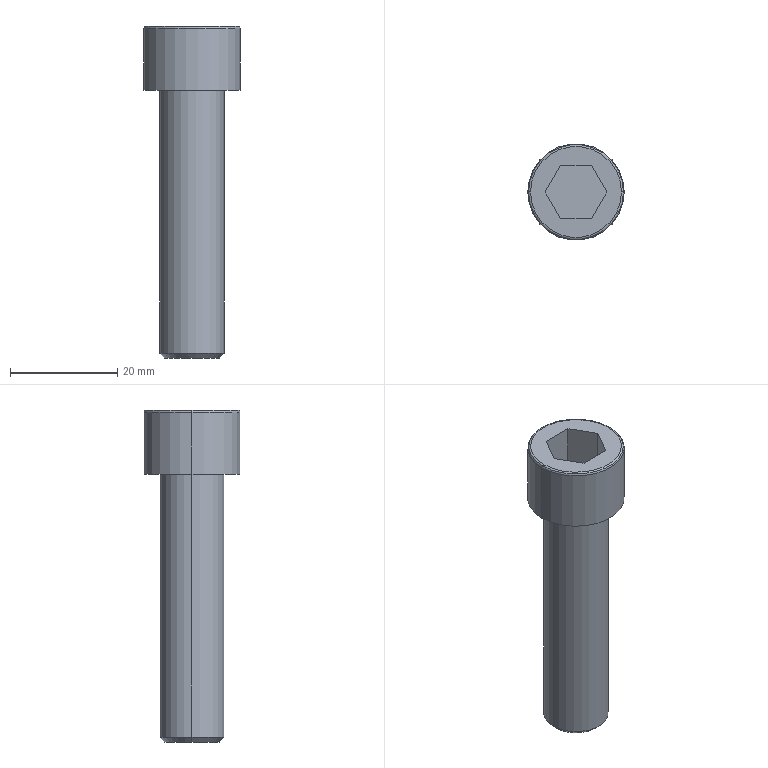Part | Creo | 1 solid | 20 faces | box 18 x 18 x 62 mm | volume 8005 mm3 | plane 10 | torus 4 | cylinder 4 | cone 2 | commonest cylinder face diameters 12 x2 18 x2
STEP:
#1=CARTESIAN_POINT('',(198.5,250.,159.5));
#2=VERTEX_POINT('',#1);
#3=CARTESIAN_POINT('',(181.5,250.,159.5));
#4=VERTEX_POINT('',#3);
#5=CARTESIAN_POINT('',(190.,250.,159.5));
#6=DIRECTION('',(0.,0.,1.));
#7=DIRECTION('',(1.,0.,0.));
#8=AXIS2_PLACEMENT_3D('',#5,#6,#7);
#9=CIRCLE('',#8,8.5);
#10=EDGE_CURVE('',#2,#4,#9,.T.);
#11=ORIENTED_EDGE('',*,*,#10,.F.);
#12=CARTESIAN_POINT('',(190.,250.,159.5));
#13=DIRECTION('',(0.,0.,1.));
#14=DIRECTION('',(-1.,0.,0.));
#15=AXIS2_PLACEMENT_3D('',#12,#13,#14);
#16=CIRCLE('',#15,8.5);
#17=EDGE_CURVE('',#4,#2,#16,.T.);
#18=ORIENTED_EDGE('',*,*,#17,.F.);
#19=EDGE_LOOP('',(#11,#18));
#20=FACE_OUTER_BOUND('',#19,.F.);
#21=CARTESIAN_POINT('',(192.887,255.,159.5));
#22=VERTEX_POINT('',#21);
#23=CARTESIAN_POINT('',(187.113,255.,159.5));
#24=VERTEX_POINT('',#23);
#25=CARTESIAN_POINT('',(192.887,255.,159.5));
#26=DIRECTION('',(-1.,0.,0.));
#27=VECTOR('',#26,5.774);
#28=LINE('',#25,#27);
#29=EDGE_CURVE('',#22,#24,#28,.T.);
#30=ORIENTED_EDGE('',*,*,#29,.T.);
#31=CARTESIAN_POINT('',(184.226,250.,159.5));
#32=VERTEX_POINT('',#31);
#33=CARTESIAN_POINT('',(184.226,250.,159.5));
#34=DIRECTION('',(0.5,0.866,0.));
#35=VECTOR('',#34,5.774);
#36=LINE('',#33,#35);
#37=EDGE_CURVE('',#32,#24,#36,.T.);
#38=ORIENTED_EDGE('',*,*,#37,.F.);
#39=CARTESIAN_POINT('',(187.113,245.,159.5));
#40=VERTEX_POINT('',#39);
#41=CARTESIAN_POINT('',(187.113,245.,159.5));
#42=DIRECTION('',(-0.5,0.866,0.));
#43=VECTOR('',#42,5.774);
#44=LINE('',#41,#43);
#45=EDGE_CURVE('',#40,#32,#44,.T.);
#46=ORIENTED_EDGE('',*,*,#45,.F.);
#47=CARTESIAN_POINT('',(192.887,245.,159.5));
#48=VERTEX_POINT('',#47);
#49=CARTESIAN_POINT('',(187.113,245.,159.5));
#50=DIRECTION('',(1.,0.,0.));
#51=VECTOR('',#50,5.774);
#52=LINE('',#49,#51);
#53=EDGE_CURVE('',#40,#48,#52,.T.);
#54=ORIENTED_EDGE('',*,*,#53,.T.);
#55=CARTESIAN_POINT('',(195.774,250.,159.5));
#56=VERTEX_POINT('',#55);
#57=CARTESIAN_POINT('',(195.774,250.,159.5));
#58=DIRECTION('',(-0.5,-0.866,0.));
#59=VECTOR('',#58,5.774);
#60=LINE('',#57,#59);
#61=EDGE_CURVE('',#56,#48,#60,.T.);
#62=ORIENTED_EDGE('',*,*,#61,.F.);
#63=CARTESIAN_POINT('',(192.887,255.,159.5));
#64=DIRECTION('',(0.5,-0.866,0.));
#65=VECTOR('',#64,5.774);
#66=LINE('',#63,#65);
#67=EDGE_CURVE('',#22,#56,#66,.T.);
#68=ORIENTED_EDGE('',*,*,#67,.F.);
#69=EDGE_LOOP('',(#30,#38,#46,#54,#62,#68));
#70=FACE_BOUND('',#69,.F.);
#71=CARTESIAN_POINT('',(190.,250.,159.5));
#72=DIRECTION('',(0.,0.,1.));
#73=DIRECTION('',(1.,0.,0.));
#74=AXIS2_PLACEMENT_3D('',#71,#72,#73);
#75=PLANE('',#74);
#76=ADVANCED_FACE('',(#20,#70),#75,.T.);
#77=ORIENTED_EDGE('',*,*,#10,.T.);
#78=CARTESIAN_POINT('',(181.146,250.,159.354));
#79=VERTEX_POINT('',#78);
#80=CARTESIAN_POINT('',(181.5,250.,159.));
#81=DIRECTION('',(0.,1.,0.));
#82=DIRECTION('',(-0.7071,0.,0.7071));
#83=AXIS2_PLACEMENT_3D('',#80,#81,#82);
#84=CIRCLE('',#83,0.5);
#85=EDGE_CURVE('',#79,#4,#84,.T.);
#86=ORIENTED_EDGE('',*,*,#85,.F.);
#87=CARTESIAN_POINT('',(198.854,250.,159.354));
#88=VERTEX_POINT('',#87);
#89=CARTESIAN_POINT('',(190.,250.,159.354));
#90=DIRECTION('',(0.,0.,1.));
#91=DIRECTION('',(1.,0.,0.));
#92=AXIS2_PLACEMENT_3D('',#89,#90,#91);
#93=CIRCLE('',#92,8.854);
#94=EDGE_CURVE('',#88,#79,#93,.T.);
#95=ORIENTED_EDGE('',*,*,#94,.F.);
#96=CARTESIAN_POINT('',(198.5,250.,159.));
#97=DIRECTION('',(0.,-1.,0.));
#98=DIRECTION('',(0.7071,0.,0.7071));
#99=AXIS2_PLACEMENT_3D('',#96,#97,#98);
#100=CIRCLE('',#99,0.5);
#101=EDGE_CURVE('',#88,#2,#100,.T.);
#102=ORIENTED_EDGE('',*,*,#101,.T.);
#103=EDGE_LOOP('',(#77,#86,#95,#102));
#104=FACE_OUTER_BOUND('',#103,.F.);
#105=CARTESIAN_POINT('',(190.,250.,159.));
#106=DIRECTION('',(0.,0.,1.));
#107=DIRECTION('',(1.,0.,0.));
#108=AXIS2_PLACEMENT_3D('',#105,#106,#107);
#109=TOROIDAL_SURFACE('',#108,8.5,0.5);
#110=ADVANCED_FACE('',(#104),#109,.T.);
#111=ORIENTED_EDGE('',*,*,#17,.T.);
#112=ORIENTED_EDGE('',*,*,#101,.F.);
#113=CARTESIAN_POINT('',(190.,250.,159.354));
#114=DIRECTION('',(0.,0.,1.));
#115=DIRECTION('',(-1.,0.,0.));
#116=AXIS2_PLACEMENT_3D('',#113,#114,#115);
#117=CIRCLE('',#116,8.854);
#118=EDGE_CURVE('',#79,#88,#117,.T.);
#119=ORIENTED_EDGE('',*,*,#118,.F.);
#120=ORIENTED_EDGE('',*,*,#85,.T.);
#121=EDGE_LOOP('',(#111,#112,#119,#120));
#122=FACE_OUTER_BOUND('',#121,.F.);
#123=CARTESIAN_POINT('',(190.,250.,159.));
#124=DIRECTION('',(0.,0.,1.));
#125=DIRECTION('',(1.,0.,0.));
#126=AXIS2_PLACEMENT_3D('',#123,#124,#125);
#127=TOROIDAL_SURFACE('',#126,8.5,0.5);
#128=ADVANCED_FACE('',(#122),#127,.T.);
#129=CARTESIAN_POINT('',(181.,250.,159.));
#130=VERTEX_POINT('',#129);
#131=CARTESIAN_POINT('',(199.,250.,159.));
#132=VERTEX_POINT('',#131);
#133=CARTESIAN_POINT('',(190.,250.,159.));
#134=DIRECTION('',(0.,0.,1.));
#135=DIRECTION('',(-1.,0.,0.));
#136=AXIS2_PLACEMENT_3D('',#133,#134,#135);
#137=CIRCLE('',#136,9.);
#138=EDGE_CURVE('',#130,#132,#137,.T.);
#139=ORIENTED_EDGE('',*,*,#138,.F.);
#140=CARTESIAN_POINT('',(181.5,250.,159.));
#141=DIRECTION('',(0.,1.,0.));
#142=DIRECTION('',(-1.,0.,0.));
#143=AXIS2_PLACEMENT_3D('',#140,#141,#142);
#144=CIRCLE('',#143,0.5);
#145=EDGE_CURVE('',#130,#79,#144,.T.);
#146=ORIENTED_EDGE('',*,*,#145,.T.);
#147=ORIENTED_EDGE('',*,*,#118,.T.);
#148=CARTESIAN_POINT('',(198.5,250.,159.));
#149=DIRECTION('',(0.,-1.,0.));
#150=DIRECTION('',(1.,0.,0.));
#151=AXIS2_PLACEMENT_3D('',#148,#149,#150);
#152=CIRCLE('',#151,0.5);
#153=EDGE_CURVE('',#132,#88,#152,.T.);
#154=ORIENTED_EDGE('',*,*,#153,.F.);
#155=EDGE_LOOP('',(#139,#146,#147,#154));
#156=FACE_OUTER_BOUND('',#155,.F.);
#157=CARTESIAN_POINT('',(190.,250.,159.));
#158=DIRECTION('',(0.,0.,1.));
#159=DIRECTION('',(1.,0.,0.));
#160=AXIS2_PLACEMENT_3D('',#157,#158,#159);
#161=TOROIDAL_SURFACE('',#160,8.5,0.5);
#162=ADVANCED_FACE('',(#156),#161,.T.);
#163=ORIENTED_EDGE('',*,*,#138,.T.);
#164=CARTESIAN_POINT('',(199.,250.,147.5));
#165=VERTEX_POINT('',#164);
#166=CARTESIAN_POINT('',(199.,250.,147.5));
#167=DIRECTION('',(0.,0.,1.));
#168=VECTOR('',#167,11.5);
#169=LINE('',#166,#168);
#170=EDGE_CURVE('',#165,#132,#169,.T.);
#171=ORIENTED_EDGE('',*,*,#170,.F.);
#172=CARTESIAN_POINT('',(181.,250.,147.5));
#173=VERTEX_POINT('',#172);
#174=CARTESIAN_POINT('',(190.,250.,147.5));
#175=DIRECTION('',(0.,0.,-1.));
#176=DIRECTION('',(1.,0.,0.));
#177=AXIS2_PLACEMENT_3D('',#174,#175,#176);
#178=CIRCLE('',#177,9.);
#179=EDGE_CURVE('',#165,#173,#178,.T.);
#180=ORIENTED_EDGE('',*,*,#179,.T.);
#181=CARTESIAN_POINT('',(181.,250.,147.5));
#182=DIRECTION('',(0.,0.,1.));
#183=VECTOR('',#182,11.5);
#184=LINE('',#181,#183);
#185=EDGE_CURVE('',#173,#130,#184,.T.);
#186=ORIENTED_EDGE('',*,*,#185,.T.);
#187=EDGE_LOOP('',(#163,#171,#180,#186));
#188=FACE_OUTER_BOUND('',#187,.F.);
#189=CARTESIAN_POINT('',(190.,250.,147.5));
#190=DIRECTION('',(0.,0.,1.));
#191=DIRECTION('',(1.,0.,0.));
#192=AXIS2_PLACEMENT_3D('',#189,#190,#191);
#193=CYLINDRICAL_SURFACE('',#192,9.);
#194=ADVANCED_FACE('',(#188),#193,.T.);
#195=CARTESIAN_POINT('',(190.,250.,159.));
#196=DIRECTION('',(0.,0.,1.));
#197=DIRECTION('',(1.,0.,0.));
#198=AXIS2_PLACEMENT_3D('',#195,#196,#197);
#199=CIRCLE('',#198,9.);
#200=EDGE_CURVE('',#132,#130,#199,.T.);
#201=ORIENTED_EDGE('',*,*,#200,.T.);
#202=ORIENTED_EDGE('',*,*,#185,.F.);
#203=CARTESIAN_POINT('',(190.,250.,147.5));
#204=DIRECTION('',(0.,0.,-1.));
#205=DIRECTION('',(-1.,0.,0.));
#206=AXIS2_PLACEMENT_3D('',#203,#204,#205);
#207=CIRCLE('',#206,9.);
#208=EDGE_CURVE('',#173,#165,#207,.T.);
#209=ORIENTED_EDGE('',*,*,#208,.T.);
#210=ORIENTED_EDGE('',*,*,#170,.T.);
#211=EDGE_LOOP('',(#201,#202,#209,#210));
#212=FACE_OUTER_BOUND('',#211,.F.);
#213=CARTESIAN_POINT('',(190.,250.,147.5));
#214=DIRECTION('',(0.,0.,1.));
#215=DIRECTION('',(1.,0.,0.));
#216=AXIS2_PLACEMENT_3D('',#213,#214,#215);
#217=CYLINDRICAL_SURFACE('',#216,9.);
#218=ADVANCED_FACE('',(#212),#217,.T.);
#219=ORIENTED_EDGE('',*,*,#200,.F.);
#220=ORIENTED_EDGE('',*,*,#153,.T.);
#221=ORIENTED_EDGE('',*,*,#94,.T.);
#222=ORIENTED_EDGE('',*,*,#145,.F.);
#223=EDGE_LOOP('',(#219,#220,#221,#222));
#224=FACE_OUTER_BOUND('',#223,.F.);
#225=CARTESIAN_POINT('',(190.,250.,159.));
#226=DIRECTION('',(0.,0.,1.));
#227=DIRECTION('',(1.,0.,0.));
#228=AXIS2_PLACEMENT_3D('',#225,#226,#227);
#229=TOROIDAL_SURFACE('',#228,8.5,0.5);
#230=ADVANCED_FACE('',(#224),#229,.T.);
#231=ORIENTED_EDGE('',*,*,#179,.F.);
#232=ORIENTED_EDGE('',*,*,#208,.F.);
#233=EDGE_LOOP('',(#231,#232));
#234=FACE_OUTER_BOUND('',#233,.F.);
#235=CARTESIAN_POINT('',(196.,250.,147.5));
#236=VERTEX_POINT('',#235);
#237=CARTESIAN_POINT('',(184.,250.,147.5));
#238=VERTEX_POINT('',#237);
#239=CARTESIAN_POINT('',(190.,250.,147.5));
#240=DIRECTION('',(0.,0.,1.));
#241=DIRECTION('',(1.,0.,0.));
#242=AXIS2_PLACEMENT_3D('',#239,#240,#241);
#243=CIRCLE('',#242,6.);
#244=EDGE_CURVE('',#236,#238,#243,.T.);
#245=ORIENTED_EDGE('',*,*,#244,.F.);
#246=CARTESIAN_POINT('',(190.,250.,147.5));
#247=DIRECTION('',(0.,0.,1.));
#248=DIRECTION('',(-1.,0.,0.));
#249=AXIS2_PLACEMENT_3D('',#246,#247,#248);
#250=CIRCLE('',#249,6.);
#251=EDGE_CURVE('',#238,#236,#250,.T.);
#252=ORIENTED_EDGE('',*,*,#251,.F.);
#253=EDGE_LOOP('',(#245,#252));
#254=FACE_BOUND('',#253,.F.);
#255=CARTESIAN_POINT('',(190.,250.,147.5));
#256=DIRECTION('',(0.,0.,-1.));
#257=DIRECTION('',(-1.,0.,0.));
#258=AXIS2_PLACEMENT_3D('',#255,#256,#257);
#259=PLANE('',#258);
#260=ADVANCED_FACE('',(#234,#254),#259,.T.);
#261=CARTESIAN_POINT('',(184.,250.,98.4));
#262=VERTEX_POINT('',#261);
#263=CARTESIAN_POINT('',(196.,250.,98.4));
#264=VERTEX_POINT('',#263);
#265=CARTESIAN_POINT('',(190.,250.,98.4));
#266=DIRECTION('',(0.,0.,-1.));
#267=DIRECTION('',(-1.,0.,0.));
#268=AXIS2_PLACEMENT_3D('',#265,#266,#267);
#269=CIRCLE('',#268,6.);
#270=EDGE_CURVE('',#262,#264,#269,.T.);
#271=ORIENTED_EDGE('',*,*,#270,.T.);
#272=CARTESIAN_POINT('',(196.,250.,98.4));
#273=DIRECTION('',(0.,0.,1.));
#274=VECTOR('',#273,49.1);
#275=LINE('',#272,#274);
#276=EDGE_CURVE('',#264,#236,#275,.T.);
#277=ORIENTED_EDGE('',*,*,#276,.T.);
#278=ORIENTED_EDGE('',*,*,#244,.T.);
#279=CARTESIAN_POINT('',(184.,250.,98.4));
#280=DIRECTION('',(0.,0.,1.));
#281=VECTOR('',#280,49.1);
#282=LINE('',#279,#281);
#283=EDGE_CURVE('',#262,#238,#282,.T.);
#284=ORIENTED_EDGE('',*,*,#283,.F.);
#285=EDGE_LOOP('',(#271,#277,#278,#284));
#286=FACE_OUTER_BOUND('',#285,.F.);
#287=CARTESIAN_POINT('',(190.,250.,97.5));
#288=DIRECTION('',(0.,0.,1.));
#289=DIRECTION('',(1.,0.,0.));
#290=AXIS2_PLACEMENT_3D('',#287,#288,#289);
#291=CYLINDRICAL_SURFACE('',#290,6.);
#292=ADVANCED_FACE('',(#286),#291,.T.);
#293=CARTESIAN_POINT('',(184.9,250.,97.5));
#294=VERTEX_POINT('',#293);
#295=CARTESIAN_POINT('',(195.1,250.,97.5));
#296=VERTEX_POINT('',#295);
#297=CARTESIAN_POINT('',(190.,250.,97.5));
#298=DIRECTION('',(0.,0.,-1.));
#299=DIRECTION('',(-1.,0.,0.));
#300=AXIS2_PLACEMENT_3D('',#297,#298,#299);
#301=CIRCLE('',#300,5.1);
#302=EDGE_CURVE('',#294,#296,#301,.T.);
#303=ORIENTED_EDGE('',*,*,#302,.T.);
#304=CARTESIAN_POINT('',(195.1,250.,97.5));
#305=DIRECTION('',(0.7071,0.,0.7071));
#306=VECTOR('',#305,1.273);
#307=LINE('',#304,#306);
#308=EDGE_CURVE('',#296,#264,#307,.T.);
#309=ORIENTED_EDGE('',*,*,#308,.T.);
#310=ORIENTED_EDGE('',*,*,#270,.F.);
#311=CARTESIAN_POINT('',(184.9,250.,97.5));
#312=DIRECTION('',(-0.7071,0.,0.7071));
#313=VECTOR('',#312,1.273);
#314=LINE('',#311,#313);
#315=EDGE_CURVE('',#294,#262,#314,.T.);
#316=ORIENTED_EDGE('',*,*,#315,.F.);
#317=EDGE_LOOP('',(#303,#309,#310,#316));
#318=FACE_OUTER_BOUND('',#317,.F.);
#319=CARTESIAN_POINT('',(190.,250.,97.95));
#320=DIRECTION('',(0.,0.,1.));
#321=DIRECTION('',(1.,0.,0.));
#322=AXIS2_PLACEMENT_3D('',#319,#320,#321);
#323=CONICAL_SURFACE('',#322,5.55,45.);
#324=ADVANCED_FACE('',(#318),#323,.T.);
#325=CARTESIAN_POINT('',(190.,250.,97.5));
#326=DIRECTION('',(0.,0.,-1.));
#327=DIRECTION('',(1.,0.,0.));
#328=AXIS2_PLACEMENT_3D('',#325,#326,#327);
#329=CIRCLE('',#328,5.1);
#330=EDGE_CURVE('',#296,#294,#329,.T.);
#331=ORIENTED_EDGE('',*,*,#330,.F.);
#332=ORIENTED_EDGE('',*,*,#302,.F.);
#333=EDGE_LOOP('',(#331,#332));
#334=FACE_OUTER_BOUND('',#333,.F.);
#335=CARTESIAN_POINT('',(190.,250.,97.5));
#336=DIRECTION('',(0.,0.,1.));
#337=DIRECTION('',(1.,0.,0.));
#338=AXIS2_PLACEMENT_3D('',#335,#336,#337);
#339=PLANE('',#338);
#340=ADVANCED_FACE('',(#334),#339,.F.);
#341=ORIENTED_EDGE('',*,*,#330,.T.);
#342=ORIENTED_EDGE('',*,*,#315,.T.);
#343=CARTESIAN_POINT('',(190.,250.,98.4));
#344=DIRECTION('',(0.,0.,-1.));
#345=DIRECTION('',(1.,0.,0.));
#346=AXIS2_PLACEMENT_3D('',#343,#344,#345);
#347=CIRCLE('',#346,6.);
#348=EDGE_CURVE('',#264,#262,#347,.T.);
#349=ORIENTED_EDGE('',*,*,#348,.F.);
#350=ORIENTED_EDGE('',*,*,#308,.F.);
#351=EDGE_LOOP('',(#341,#342,#349,#350));
#352=FACE_OUTER_BOUND('',#351,.F.);
#353=CARTESIAN_POINT('',(190.,250.,97.95));
#354=DIRECTION('',(0.,0.,1.));
#355=DIRECTION('',(1.,0.,0.));
#356=AXIS2_PLACEMENT_3D('',#353,#354,#355);
#357=CONICAL_SURFACE('',#356,5.55,45.);
#358=ADVANCED_FACE('',(#352),#357,.T.);
#359=ORIENTED_EDGE('',*,*,#348,.T.);
#360=ORIENTED_EDGE('',*,*,#283,.T.);
#361=ORIENTED_EDGE('',*,*,#251,.T.);
#362=ORIENTED_EDGE('',*,*,#276,.F.);
#363=EDGE_LOOP('',(#359,#360,#361,#362));
#364=FACE_OUTER_BOUND('',#363,.F.);
#365=CARTESIAN_POINT('',(190.,250.,97.5));
#366=DIRECTION('',(0.,0.,1.));
#367=DIRECTION('',(1.,0.,0.));
#368=AXIS2_PLACEMENT_3D('',#365,#366,#367);
#369=CYLINDRICAL_SURFACE('',#368,6.);
#370=ADVANCED_FACE('',(#364),#369,.T.);
#371=ORIENTED_EDGE('',*,*,#29,.F.);
#372=CARTESIAN_POINT('',(192.887,255.,151.58));
#373=VERTEX_POINT('',#372);
#374=CARTESIAN_POINT('',(192.887,255.,159.5));
#375=DIRECTION('',(0.,0.,-1.));
#376=VECTOR('',#375,7.92);
#377=LINE('',#374,#376);
#378=EDGE_CURVE('',#22,#373,#377,.T.);
#379=ORIENTED_EDGE('',*,*,#378,.T.);
#380=CARTESIAN_POINT('',(187.113,255.,151.58));
#381=VERTEX_POINT('',#380);
#382=CARTESIAN_POINT('',(192.887,255.,151.58));
#383=DIRECTION('',(-1.,0.,0.));
#384=VECTOR('',#383,5.774);
#385=LINE('',#382,#384);
#386=EDGE_CURVE('',#373,#381,#385,.T.);
#387=ORIENTED_EDGE('',*,*,#386,.T.);
#388=CARTESIAN_POINT('',(187.113,255.,159.5));
#389=DIRECTION('',(0.,0.,-1.));
#390=VECTOR('',#389,7.92);
#391=LINE('',#388,#390);
#392=EDGE_CURVE('',#24,#381,#391,.T.);
#393=ORIENTED_EDGE('',*,*,#392,.F.);
#394=EDGE_LOOP('',(#371,#379,#387,#393));
#395=FACE_OUTER_BOUND('',#394,.F.);
#396=CARTESIAN_POINT('',(187.113,255.,151.58));
#397=DIRECTION('',(0.,-1.,0.));
#398=DIRECTION('',(0.,0.,-1.));
#399=AXIS2_PLACEMENT_3D('',#396,#397,#398);
#400=PLANE('',#399);
#401=ADVANCED_FACE('',(#395),#400,.T.);
#402=ORIENTED_EDGE('',*,*,#67,.T.);
#403=CARTESIAN_POINT('',(195.774,250.,151.58));
#404=VERTEX_POINT('',#403);
#405=CARTESIAN_POINT('',(195.774,250.,159.5));
#406=DIRECTION('',(0.,0.,-1.));
#407=VECTOR('',#406,7.92);
#408=LINE('',#405,#407);
#409=EDGE_CURVE('',#56,#404,#408,.T.);
#410=ORIENTED_EDGE('',*,*,#409,.T.);
#411=CARTESIAN_POINT('',(195.774,250.,151.58));
#412=DIRECTION('',(-0.5,0.866,0.));
#413=VECTOR('',#412,5.774);
#414=LINE('',#411,#413);
#415=EDGE_CURVE('',#404,#373,#414,.T.);
#416=ORIENTED_EDGE('',*,*,#415,.T.);
#417=ORIENTED_EDGE('',*,*,#378,.F.);
#418=EDGE_LOOP('',(#402,#410,#416,#417));
#419=FACE_OUTER_BOUND('',#418,.F.);
#420=CARTESIAN_POINT('',(192.887,255.,151.58));
#421=DIRECTION('',(-0.866,-0.5,0.));
#422=DIRECTION('',(0.5,-0.866,0.));
#423=AXIS2_PLACEMENT_3D('',#420,#421,#422);
#424=PLANE('',#423);
#425=ADVANCED_FACE('',(#419),#424,.T.);
#426=ORIENTED_EDGE('',*,*,#61,.T.);
#427=CARTESIAN_POINT('',(192.887,245.,151.58));
#428=VERTEX_POINT('',#427);
#429=CARTESIAN_POINT('',(192.887,245.,159.5));
#430=DIRECTION('',(0.,0.,-1.));
#431=VECTOR('',#430,7.92);
#432=LINE('',#429,#431);
#433=EDGE_CURVE('',#48,#428,#432,.T.);
#434=ORIENTED_EDGE('',*,*,#433,.T.);
#435=CARTESIAN_POINT('',(192.887,245.,151.58));
#436=DIRECTION('',(0.5,0.866,0.));
#437=VECTOR('',#436,5.774);
#438=LINE('',#435,#437);
#439=EDGE_CURVE('',#428,#404,#438,.T.);
#440=ORIENTED_EDGE('',*,*,#439,.T.);
#441=ORIENTED_EDGE('',*,*,#409,.F.);
#442=EDGE_LOOP('',(#426,#434,#440,#441));
#443=FACE_OUTER_BOUND('',#442,.F.);
#444=CARTESIAN_POINT('',(195.774,250.,151.58));
#445=DIRECTION('',(-0.866,0.5,0.));
#446=DIRECTION('',(-0.5,-0.866,0.));
#447=AXIS2_PLACEMENT_3D('',#444,#445,#446);
#448=PLANE('',#447);
#449=ADVANCED_FACE('',(#443),#448,.T.);
#450=ORIENTED_EDGE('',*,*,#53,.F.);
#451=CARTESIAN_POINT('',(187.113,245.,151.58));
#452=VERTEX_POINT('',#451);
#453=CARTESIAN_POINT('',(187.113,245.,159.5));
#454=DIRECTION('',(0.,0.,-1.));
#455=VECTOR('',#454,7.92);
#456=LINE('',#453,#455);
#457=EDGE_CURVE('',#40,#452,#456,.T.);
#458=ORIENTED_EDGE('',*,*,#457,.T.);
#459=CARTESIAN_POINT('',(187.113,245.,151.58));
#460=DIRECTION('',(1.,0.,0.));
#461=VECTOR('',#460,5.774);
#462=LINE('',#459,#461);
#463=EDGE_CURVE('',#452,#428,#462,.T.);
#464=ORIENTED_EDGE('',*,*,#463,.T.);
#465=ORIENTED_EDGE('',*,*,#433,.F.);
#466=EDGE_LOOP('',(#450,#458,#464,#465));
#467=FACE_OUTER_BOUND('',#466,.F.);
#468=CARTESIAN_POINT('',(192.887,245.,151.58));
#469=DIRECTION('',(0.,1.,0.));
#470=DIRECTION('',(0.,0.,1.));
#471=AXIS2_PLACEMENT_3D('',#468,#469,#470);
#472=PLANE('',#471);
#473=ADVANCED_FACE('',(#467),#472,.T.);
#474=ORIENTED_EDGE('',*,*,#45,.T.);
#475=CARTESIAN_POINT('',(184.226,250.,151.58));
#476=VERTEX_POINT('',#475);
#477=CARTESIAN_POINT('',(184.226,250.,159.5));
#478=DIRECTION('',(0.,0.,-1.));
#479=VECTOR('',#478,7.92);
#480=LINE('',#477,#479);
#481=EDGE_CURVE('',#32,#476,#480,.T.);
#482=ORIENTED_EDGE('',*,*,#481,.T.);
#483=CARTESIAN_POINT('',(184.226,250.,151.58));
#484=DIRECTION('',(0.5,-0.866,0.));
#485=VECTOR('',#484,5.774);
#486=LINE('',#483,#485);
#487=EDGE_CURVE('',#476,#452,#486,.T.);
#488=ORIENTED_EDGE('',*,*,#487,.T.);
#489=ORIENTED_EDGE('',*,*,#457,.F.);
#490=EDGE_LOOP('',(#474,#482,#488,#489));
#491=FACE_OUTER_BOUND('',#490,.F.);
#492=CARTESIAN_POINT('',(187.113,245.,151.58));
#493=DIRECTION('',(0.866,0.5,0.));
#494=DIRECTION('',(-0.5,0.866,0.));
#495=AXIS2_PLACEMENT_3D('',#492,#493,#494);
#496=PLANE('',#495);
#497=ADVANCED_FACE('',(#491),#496,.T.);
#498=ORIENTED_EDGE('',*,*,#37,.T.);
#499=ORIENTED_EDGE('',*,*,#392,.T.);
#500=CARTESIAN_POINT('',(187.113,255.,151.58));
#501=DIRECTION('',(-0.5,-0.866,0.));
#502=VECTOR('',#501,5.774);
#503=LINE('',#500,#502);
#504=EDGE_CURVE('',#381,#476,#503,.T.);
#505=ORIENTED_EDGE('',*,*,#504,.T.);
#506=ORIENTED_EDGE('',*,*,#481,.F.);
#507=EDGE_LOOP('',(#498,#499,#505,#506));
#508=FACE_OUTER_BOUND('',#507,.F.);
#509=CARTESIAN_POINT('',(184.226,250.,151.58));
#510=DIRECTION('',(0.866,-0.5,0.));
#511=DIRECTION('',(0.5,0.866,0.));
#512=AXIS2_PLACEMENT_3D('',#509,#510,#511);
#513=PLANE('',#512);
#514=ADVANCED_FACE('',(#508),#513,.T.);
#515=ORIENTED_EDGE('',*,*,#415,.F.);
#516=ORIENTED_EDGE('',*,*,#439,.F.);
#517=ORIENTED_EDGE('',*,*,#463,.F.);
#518=ORIENTED_EDGE('',*,*,#487,.F.);
#519=ORIENTED_EDGE('',*,*,#504,.F.);
#520=ORIENTED_EDGE('',*,*,#386,.F.);
#521=EDGE_LOOP('',(#515,#516,#517,#518,#519,#520));
#522=FACE_OUTER_BOUND('',#521,.F.);
#523=CARTESIAN_POINT('',(198.66,245.,151.58));
#524=DIRECTION('',(0.,0.,-1.));
#525=DIRECTION('',(-1.,0.,0.));
#526=AXIS2_PLACEMENT_3D('',#523,#524,#525);
#527=PLANE('',#526);
#528=ADVANCED_FACE('',(#522),#527,.F.);
#529=CLOSED_SHELL('',(#76,#110,#128,#162,#194,#218,#230,#260,#292,#324,#340,#358,#370,#401,#425,#449,#473,#497,#514,#528));
#530=MANIFOLD_SOLID_BREP('',#529);
#531=(LENGTH_UNIT()NAMED_UNIT(*)SI_UNIT(.MILLI.,.METRE.));
#532=UNCERTAINTY_MEASURE_WITH_UNIT(LENGTH_MEASURE(0.006702),#531,'','');
#533=(NAMED_UNIT(*)PLANE_ANGLE_UNIT()SI_UNIT($,.RADIAN.));
#534=PLANE_ANGLE_MEASURE_WITH_UNIT(PLANE_ANGLE_MEASURE(0.01745),#533);
#535=(CONVERSION_BASED_UNIT('DEGREE',#534)NAMED_UNIT(*)PLANE_ANGLE_UNIT());
#536=(NAMED_UNIT(*)SI_UNIT($,.STERADIAN.)SOLID_ANGLE_UNIT());
#537=(GEOMETRIC_REPRESENTATION_CONTEXT(3)GLOBAL_UNCERTAINTY_ASSIGNED_CONTEXT((#532))GLOBAL_UNIT_ASSIGNED_CONTEXT((#531,#535,#536))REPRESENTATION_CONTEXT('',''));
#538=ADVANCED_BREP_SHAPE_REPRESENTATION('',(#530),#537);